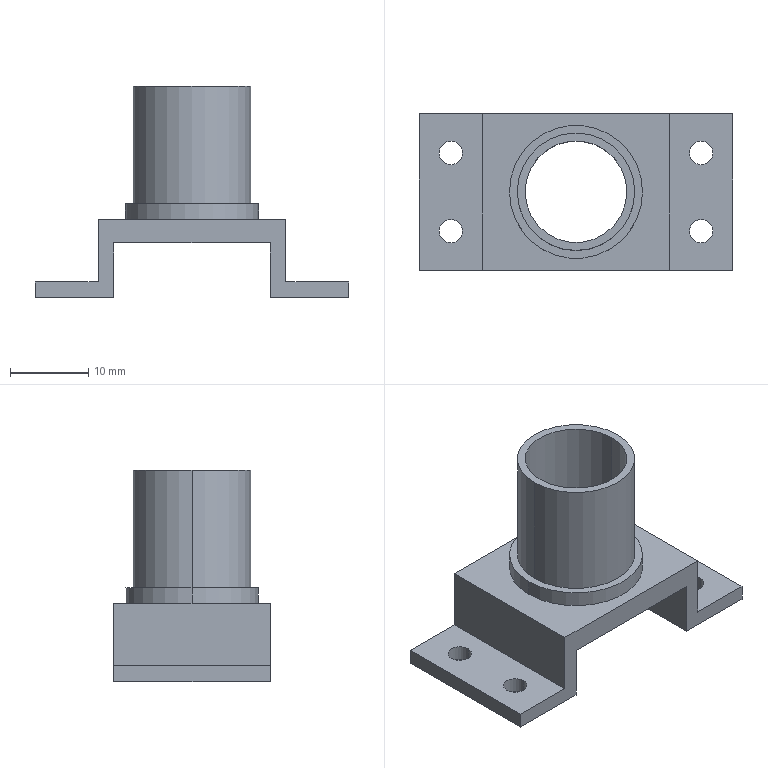Part | SolidWorks | features ICE 9, Extrusion 1 | 1 solid | 30 faces | box 40 x 20 x 27 mm | volume 3033 mm3 | plane 16 | cylinder 14 | commonest cylinder face diameters 3 x8 13 x2 15 x2 17 x2
STEP:
#1=CARTESIAN_POINT('',(14.5,-5.,-5.));
#2=VERTEX_POINT('',#1);
#3=CARTESIAN_POINT('',(17.5,-5.,-5.));
#4=VERTEX_POINT('',#3);
#5=CARTESIAN_POINT('',(16.,-5.,-5.));
#6=DIRECTION('',(0.,0.,1.));
#7=DIRECTION('',(1.,0.,0.));
#8=AXIS2_PLACEMENT_3D('',#5,#6,#7);
#9=CIRCLE('',#8,1.5);
#10=EDGE_CURVE('',#2,#4,#9,.T.);
#11=ORIENTED_EDGE('',*,*,#10,.F.);
#12=CARTESIAN_POINT('',(14.5,-5.,-3.));
#13=VERTEX_POINT('',#12);
#14=CARTESIAN_POINT('',(14.5,-5.,-5.));
#15=DIRECTION('',(0.,0.,1.));
#16=VECTOR('',#15,1000.);
#17=LINE('',#14,#16);
#18=EDGE_CURVE('',#2,#13,#17,.T.);
#19=ORIENTED_EDGE('',*,*,#18,.T.);
#20=CARTESIAN_POINT('',(17.5,-5.,-3.));
#21=VERTEX_POINT('',#20);
#22=CARTESIAN_POINT('',(16.,-5.,-3.));
#23=DIRECTION('',(0.,0.,1.));
#24=DIRECTION('',(1.,0.,0.));
#25=AXIS2_PLACEMENT_3D('',#22,#23,#24);
#26=CIRCLE('',#25,1.5);
#27=EDGE_CURVE('',#13,#21,#26,.T.);
#28=ORIENTED_EDGE('',*,*,#27,.T.);
#29=CARTESIAN_POINT('',(17.5,-5.,-5.));
#30=DIRECTION('',(0.,0.,1.));
#31=VECTOR('',#30,1000.);
#32=LINE('',#29,#31);
#33=EDGE_CURVE('',#4,#21,#32,.T.);
#34=ORIENTED_EDGE('',*,*,#33,.F.);
#35=EDGE_LOOP('',(#11,#19,#28,#34));
#36=FACE_OUTER_BOUND('',#35,.T.);
#37=CARTESIAN_POINT('',(16.,-5.,-5.));
#38=DIRECTION('',(0.,0.,1.));
#39=DIRECTION('',(1.,0.,0.));
#40=AXIS2_PLACEMENT_3D('',#37,#38,#39);
#41=CYLINDRICAL_SURFACE('',#40,1.5);
#42=ADVANCED_FACE('',(#36),#41,.F.);
#43=CARTESIAN_POINT('',(14.5,5.,-5.));
#44=VERTEX_POINT('',#43);
#45=CARTESIAN_POINT('',(17.5,5.,-5.));
#46=VERTEX_POINT('',#45);
#47=CARTESIAN_POINT('',(16.,5.,-5.));
#48=DIRECTION('',(0.,0.,1.));
#49=DIRECTION('',(1.,0.,0.));
#50=AXIS2_PLACEMENT_3D('',#47,#48,#49);
#51=CIRCLE('',#50,1.5);
#52=EDGE_CURVE('',#44,#46,#51,.T.);
#53=ORIENTED_EDGE('',*,*,#52,.F.);
#54=CARTESIAN_POINT('',(14.5,5.,-3.));
#55=VERTEX_POINT('',#54);
#56=CARTESIAN_POINT('',(14.5,5.,-5.));
#57=DIRECTION('',(0.,0.,1.));
#58=VECTOR('',#57,1000.);
#59=LINE('',#56,#58);
#60=EDGE_CURVE('',#44,#55,#59,.T.);
#61=ORIENTED_EDGE('',*,*,#60,.T.);
#62=CARTESIAN_POINT('',(17.5,5.,-3.));
#63=VERTEX_POINT('',#62);
#64=CARTESIAN_POINT('',(16.,5.,-3.));
#65=DIRECTION('',(0.,0.,1.));
#66=DIRECTION('',(1.,0.,0.));
#67=AXIS2_PLACEMENT_3D('',#64,#65,#66);
#68=CIRCLE('',#67,1.5);
#69=EDGE_CURVE('',#55,#63,#68,.T.);
#70=ORIENTED_EDGE('',*,*,#69,.T.);
#71=CARTESIAN_POINT('',(17.5,5.,-5.));
#72=DIRECTION('',(0.,0.,1.));
#73=VECTOR('',#72,1000.);
#74=LINE('',#71,#73);
#75=EDGE_CURVE('',#46,#63,#74,.T.);
#76=ORIENTED_EDGE('',*,*,#75,.F.);
#77=EDGE_LOOP('',(#53,#61,#70,#76));
#78=FACE_OUTER_BOUND('',#77,.T.);
#79=CARTESIAN_POINT('',(16.,5.,-5.));
#80=DIRECTION('',(0.,0.,1.));
#81=DIRECTION('',(1.,0.,0.));
#82=AXIS2_PLACEMENT_3D('',#79,#80,#81);
#83=CYLINDRICAL_SURFACE('',#82,1.5);
#84=ADVANCED_FACE('',(#78),#83,.F.);
#85=CARTESIAN_POINT('',(-17.5,5.,-5.));
#86=VERTEX_POINT('',#85);
#87=CARTESIAN_POINT('',(-14.5,5.,-5.));
#88=VERTEX_POINT('',#87);
#89=CARTESIAN_POINT('',(-16.,5.,-5.));
#90=DIRECTION('',(0.,0.,1.));
#91=DIRECTION('',(-1.,0.,0.));
#92=AXIS2_PLACEMENT_3D('',#89,#90,#91);
#93=CIRCLE('',#92,1.5);
#94=EDGE_CURVE('',#86,#88,#93,.T.);
#95=ORIENTED_EDGE('',*,*,#94,.F.);
#96=CARTESIAN_POINT('',(-17.5,5.,-3.));
#97=VERTEX_POINT('',#96);
#98=CARTESIAN_POINT('',(-17.5,5.,-5.));
#99=DIRECTION('',(0.,0.,1.));
#100=VECTOR('',#99,1000.);
#101=LINE('',#98,#100);
#102=EDGE_CURVE('',#86,#97,#101,.T.);
#103=ORIENTED_EDGE('',*,*,#102,.T.);
#104=CARTESIAN_POINT('',(-14.5,5.,-3.));
#105=VERTEX_POINT('',#104);
#106=CARTESIAN_POINT('',(-16.,5.,-3.));
#107=DIRECTION('',(0.,0.,1.));
#108=DIRECTION('',(-1.,0.,0.));
#109=AXIS2_PLACEMENT_3D('',#106,#107,#108);
#110=CIRCLE('',#109,1.5);
#111=EDGE_CURVE('',#97,#105,#110,.T.);
#112=ORIENTED_EDGE('',*,*,#111,.T.);
#113=CARTESIAN_POINT('',(-14.5,5.,-5.));
#114=DIRECTION('',(0.,0.,1.));
#115=VECTOR('',#114,1000.);
#116=LINE('',#113,#115);
#117=EDGE_CURVE('',#88,#105,#116,.T.);
#118=ORIENTED_EDGE('',*,*,#117,.F.);
#119=EDGE_LOOP('',(#95,#103,#112,#118));
#120=FACE_OUTER_BOUND('',#119,.T.);
#121=CARTESIAN_POINT('',(-16.,5.,-5.));
#122=DIRECTION('',(0.,0.,1.));
#123=DIRECTION('',(1.,0.,0.));
#124=AXIS2_PLACEMENT_3D('',#121,#122,#123);
#125=CYLINDRICAL_SURFACE('',#124,1.5);
#126=ADVANCED_FACE('',(#120),#125,.F.);
#127=CARTESIAN_POINT('',(-17.5,-5.,-5.));
#128=VERTEX_POINT('',#127);
#129=CARTESIAN_POINT('',(-14.5,-5.,-5.));
#130=VERTEX_POINT('',#129);
#131=CARTESIAN_POINT('',(-16.,-5.,-5.));
#132=DIRECTION('',(0.,0.,1.));
#133=DIRECTION('',(-1.,0.,0.));
#134=AXIS2_PLACEMENT_3D('',#131,#132,#133);
#135=CIRCLE('',#134,1.5);
#136=EDGE_CURVE('',#128,#130,#135,.T.);
#137=ORIENTED_EDGE('',*,*,#136,.F.);
#138=CARTESIAN_POINT('',(-17.5,-5.,-3.));
#139=VERTEX_POINT('',#138);
#140=CARTESIAN_POINT('',(-17.5,-5.,-5.));
#141=DIRECTION('',(0.,0.,1.));
#142=VECTOR('',#141,1000.);
#143=LINE('',#140,#142);
#144=EDGE_CURVE('',#128,#139,#143,.T.);
#145=ORIENTED_EDGE('',*,*,#144,.T.);
#146=CARTESIAN_POINT('',(-14.5,-5.,-3.));
#147=VERTEX_POINT('',#146);
#148=CARTESIAN_POINT('',(-16.,-5.,-3.));
#149=DIRECTION('',(0.,0.,1.));
#150=DIRECTION('',(-1.,0.,0.));
#151=AXIS2_PLACEMENT_3D('',#148,#149,#150);
#152=CIRCLE('',#151,1.5);
#153=EDGE_CURVE('',#139,#147,#152,.T.);
#154=ORIENTED_EDGE('',*,*,#153,.T.);
#155=CARTESIAN_POINT('',(-14.5,-5.,-5.));
#156=DIRECTION('',(0.,0.,1.));
#157=VECTOR('',#156,1000.);
#158=LINE('',#155,#157);
#159=EDGE_CURVE('',#130,#147,#158,.T.);
#160=ORIENTED_EDGE('',*,*,#159,.F.);
#161=EDGE_LOOP('',(#137,#145,#154,#160));
#162=FACE_OUTER_BOUND('',#161,.T.);
#163=CARTESIAN_POINT('',(-16.,-5.,-5.));
#164=DIRECTION('',(0.,0.,1.));
#165=DIRECTION('',(1.,0.,0.));
#166=AXIS2_PLACEMENT_3D('',#163,#164,#165);
#167=CYLINDRICAL_SURFACE('',#166,1.5);
#168=ADVANCED_FACE('',(#162),#167,.F.);
#169=CARTESIAN_POINT('',(-8.5,0.,5.));
#170=VERTEX_POINT('',#169);
#171=CARTESIAN_POINT('',(8.5,0.,5.));
#172=VERTEX_POINT('',#171);
#173=CARTESIAN_POINT('',(0.,0.,5.));
#174=DIRECTION('',(0.,0.,-1.));
#175=DIRECTION('',(-1.,0.,0.));
#176=AXIS2_PLACEMENT_3D('',#173,#174,#175);
#177=CIRCLE('',#176,8.5);
#178=EDGE_CURVE('',#170,#172,#177,.T.);
#179=ORIENTED_EDGE('',*,*,#178,.F.);
#180=CARTESIAN_POINT('',(-8.5,0.,7.));
#181=VERTEX_POINT('',#180);
#182=CARTESIAN_POINT('',(-8.5,0.,5.));
#183=DIRECTION('',(0.,0.,1.));
#184=VECTOR('',#183,1000.);
#185=LINE('',#182,#184);
#186=EDGE_CURVE('',#170,#181,#185,.T.);
#187=ORIENTED_EDGE('',*,*,#186,.T.);
#188=CARTESIAN_POINT('',(8.5,0.,7.));
#189=VERTEX_POINT('',#188);
#190=CARTESIAN_POINT('',(0.,0.,7.));
#191=DIRECTION('',(0.,0.,-1.));
#192=DIRECTION('',(-1.,0.,0.));
#193=AXIS2_PLACEMENT_3D('',#190,#191,#192);
#194=CIRCLE('',#193,8.5);
#195=EDGE_CURVE('',#181,#189,#194,.T.);
#196=ORIENTED_EDGE('',*,*,#195,.T.);
#197=CARTESIAN_POINT('',(8.5,0.,5.));
#198=DIRECTION('',(0.,0.,1.));
#199=VECTOR('',#198,1000.);
#200=LINE('',#197,#199);
#201=EDGE_CURVE('',#172,#189,#200,.T.);
#202=ORIENTED_EDGE('',*,*,#201,.F.);
#203=EDGE_LOOP('',(#179,#187,#196,#202));
#204=FACE_OUTER_BOUND('',#203,.T.);
#205=CARTESIAN_POINT('',(0.,0.,5.));
#206=DIRECTION('',(0.,0.,1.));
#207=DIRECTION('',(1.,0.,0.));
#208=AXIS2_PLACEMENT_3D('',#205,#206,#207);
#209=CYLINDRICAL_SURFACE('',#208,8.5);
#210=ADVANCED_FACE('',(#204),#209,.T.);
#211=CARTESIAN_POINT('',(7.5,0.,22.));
#212=VERTEX_POINT('',#211);
#213=CARTESIAN_POINT('',(-7.5,0.,22.));
#214=VERTEX_POINT('',#213);
#215=CARTESIAN_POINT('',(0.,0.,22.));
#216=DIRECTION('',(0.,0.,1.));
#217=DIRECTION('',(1.,0.,0.));
#218=AXIS2_PLACEMENT_3D('',#215,#216,#217);
#219=CIRCLE('',#218,7.5);
#220=EDGE_CURVE('',#212,#214,#219,.T.);
#221=ORIENTED_EDGE('',*,*,#220,.F.);
#222=CARTESIAN_POINT('',(7.5,0.,7.));
#223=VERTEX_POINT('',#222);
#224=CARTESIAN_POINT('',(7.5,0.,22.));
#225=DIRECTION('',(0.,0.,-1.));
#226=VECTOR('',#225,1000.);
#227=LINE('',#224,#226);
#228=EDGE_CURVE('',#212,#223,#227,.T.);
#229=ORIENTED_EDGE('',*,*,#228,.T.);
#230=CARTESIAN_POINT('',(-7.5,0.,7.));
#231=VERTEX_POINT('',#230);
#232=CARTESIAN_POINT('',(0.,0.,7.));
#233=DIRECTION('',(0.,0.,-1.));
#234=DIRECTION('',(-1.,0.,0.));
#235=AXIS2_PLACEMENT_3D('',#232,#233,#234);
#236=CIRCLE('',#235,7.5);
#237=EDGE_CURVE('',#231,#223,#236,.T.);
#238=ORIENTED_EDGE('',*,*,#237,.F.);
#239=CARTESIAN_POINT('',(-7.5,0.,22.));
#240=DIRECTION('',(0.,0.,-1.));
#241=VECTOR('',#240,1000.);
#242=LINE('',#239,#241);
#243=EDGE_CURVE('',#214,#231,#242,.T.);
#244=ORIENTED_EDGE('',*,*,#243,.F.);
#245=EDGE_LOOP('',(#221,#229,#238,#244));
#246=FACE_OUTER_BOUND('',#245,.T.);
#247=CARTESIAN_POINT('',(0.,0.,22.));
#248=DIRECTION('',(0.,0.,-1.));
#249=DIRECTION('',(-1.,0.,0.));
#250=AXIS2_PLACEMENT_3D('',#247,#248,#249);
#251=CYLINDRICAL_SURFACE('',#250,7.5);
#252=ADVANCED_FACE('',(#246),#251,.T.);
#253=CARTESIAN_POINT('',(-6.5,0.,22.));
#254=VERTEX_POINT('',#253);
#255=CARTESIAN_POINT('',(6.5,0.,22.));
#256=VERTEX_POINT('',#255);
#257=CARTESIAN_POINT('',(0.,0.,22.));
#258=DIRECTION('',(0.,0.,1.));
#259=DIRECTION('',(1.,0.,0.));
#260=AXIS2_PLACEMENT_3D('',#257,#258,#259);
#261=CIRCLE('',#260,6.5);
#262=EDGE_CURVE('',#254,#256,#261,.T.);
#263=ORIENTED_EDGE('',*,*,#262,.T.);
#264=CARTESIAN_POINT('',(6.5,0.,2.));
#265=VERTEX_POINT('',#264);
#266=CARTESIAN_POINT('',(6.5,0.,22.));
#267=DIRECTION('',(0.,0.,-1.));
#268=VECTOR('',#267,1000.);
#269=LINE('',#266,#268);
#270=EDGE_CURVE('',#256,#265,#269,.T.);
#271=ORIENTED_EDGE('',*,*,#270,.T.);
#272=CARTESIAN_POINT('',(-6.5,0.,2.));
#273=VERTEX_POINT('',#272);
#274=CARTESIAN_POINT('',(0.,0.,2.));
#275=DIRECTION('',(0.,0.,-1.));
#276=DIRECTION('',(-1.,0.,0.));
#277=AXIS2_PLACEMENT_3D('',#274,#275,#276);
#278=CIRCLE('',#277,6.5);
#279=EDGE_CURVE('',#265,#273,#278,.T.);
#280=ORIENTED_EDGE('',*,*,#279,.T.);
#281=CARTESIAN_POINT('',(-6.5,0.,22.));
#282=DIRECTION('',(0.,0.,-1.));
#283=VECTOR('',#282,1000.);
#284=LINE('',#281,#283);
#285=EDGE_CURVE('',#254,#273,#284,.T.);
#286=ORIENTED_EDGE('',*,*,#285,.F.);
#287=EDGE_LOOP('',(#263,#271,#280,#286));
#288=FACE_OUTER_BOUND('',#287,.T.);
#289=CARTESIAN_POINT('',(0.,0.,22.));
#290=DIRECTION('',(0.,0.,-1.));
#291=DIRECTION('',(-1.,0.,0.));
#292=AXIS2_PLACEMENT_3D('',#289,#290,#291);
#293=CYLINDRICAL_SURFACE('',#292,6.5);
#294=ADVANCED_FACE('',(#288),#293,.F.);
#295=CARTESIAN_POINT('',(-16.,5.,-5.));
#296=DIRECTION('',(0.,0.,1.));
#297=DIRECTION('',(-1.,0.,0.));
#298=AXIS2_PLACEMENT_3D('',#295,#296,#297);
#299=CIRCLE('',#298,1.5);
#300=EDGE_CURVE('',#88,#86,#299,.T.);
#301=ORIENTED_EDGE('',*,*,#300,.T.);
#302=ORIENTED_EDGE('',*,*,#94,.T.);
#303=EDGE_LOOP('',(#301,#302));
#304=FACE_BOUND('',#303,.T.);
#305=CARTESIAN_POINT('',(-16.,-5.,-5.));
#306=DIRECTION('',(0.,0.,1.));
#307=DIRECTION('',(-1.,0.,0.));
#308=AXIS2_PLACEMENT_3D('',#305,#306,#307);
#309=CIRCLE('',#308,1.5);
#310=EDGE_CURVE('',#130,#128,#309,.T.);
#311=ORIENTED_EDGE('',*,*,#310,.T.);
#312=ORIENTED_EDGE('',*,*,#136,.T.);
#313=EDGE_LOOP('',(#311,#312));
#314=FACE_BOUND('',#313,.T.);
#315=CARTESIAN_POINT('',(-10.,10.,-5.));
#316=VERTEX_POINT('',#315);
#317=CARTESIAN_POINT('',(-10.,-10.,-5.));
#318=VERTEX_POINT('',#317);
#319=CARTESIAN_POINT('',(-10.,10.,-5.));
#320=DIRECTION('',(0.,-1.,0.));
#321=VECTOR('',#320,1000.);
#322=LINE('',#319,#321);
#323=EDGE_CURVE('',#316,#318,#322,.T.);
#324=ORIENTED_EDGE('',*,*,#323,.T.);
#325=CARTESIAN_POINT('',(-20.,-10.,-5.));
#326=VERTEX_POINT('',#325);
#327=CARTESIAN_POINT('',(-15.,-10.,-5.));
#328=DIRECTION('',(-1.,0.,0.));
#329=VECTOR('',#328,1000.);
#330=LINE('',#327,#329);
#331=EDGE_CURVE('',#318,#326,#330,.T.);
#332=ORIENTED_EDGE('',*,*,#331,.T.);
#333=CARTESIAN_POINT('',(-20.,10.,-5.));
#334=VERTEX_POINT('',#333);
#335=CARTESIAN_POINT('',(-20.,10.,-5.));
#336=DIRECTION('',(0.,1.,0.));
#337=VECTOR('',#336,1000.);
#338=LINE('',#335,#337);
#339=EDGE_CURVE('',#326,#334,#338,.T.);
#340=ORIENTED_EDGE('',*,*,#339,.T.);
#341=CARTESIAN_POINT('',(-15.,10.,-5.));
#342=DIRECTION('',(1.,0.,0.));
#343=VECTOR('',#342,1000.);
#344=LINE('',#341,#343);
#345=EDGE_CURVE('',#334,#316,#344,.T.);
#346=ORIENTED_EDGE('',*,*,#345,.T.);
#347=EDGE_LOOP('',(#324,#332,#340,#346));
#348=FACE_OUTER_BOUND('',#347,.T.);
#349=CARTESIAN_POINT('',(0.,0.,-5.));
#350=DIRECTION('',(0.,0.,-1.));
#351=DIRECTION('',(-1.,0.,0.));
#352=AXIS2_PLACEMENT_3D('',#349,#350,#351);
#353=PLANE('',#352);
#354=ADVANCED_FACE('',(#304,#314,#348),#353,.T.);
#355=CARTESIAN_POINT('',(12.,-10.,5.));
#356=VERTEX_POINT('',#355);
#357=CARTESIAN_POINT('',(-12.,-10.,5.));
#358=VERTEX_POINT('',#357);
#359=CARTESIAN_POINT('',(-15.,-10.,5.));
#360=DIRECTION('',(-1.,0.,0.));
#361=VECTOR('',#360,1000.);
#362=LINE('',#359,#361);
#363=EDGE_CURVE('',#356,#358,#362,.T.);
#364=ORIENTED_EDGE('',*,*,#363,.T.);
#365=CARTESIAN_POINT('',(-12.,-10.,-3.));
#366=VERTEX_POINT('',#365);
#367=CARTESIAN_POINT('',(-12.,-10.,-3.));
#368=DIRECTION('',(0.,0.,1.));
#369=VECTOR('',#368,1000.);
#370=LINE('',#367,#369);
#371=EDGE_CURVE('',#366,#358,#370,.T.);
#372=ORIENTED_EDGE('',*,*,#371,.F.);
#373=CARTESIAN_POINT('',(-20.,-10.,-3.));
#374=VERTEX_POINT('',#373);
#375=CARTESIAN_POINT('',(-15.,-10.,-3.));
#376=DIRECTION('',(-1.,0.,0.));
#377=VECTOR('',#376,1000.);
#378=LINE('',#375,#377);
#379=EDGE_CURVE('',#366,#374,#378,.T.);
#380=ORIENTED_EDGE('',*,*,#379,.T.);
#381=CARTESIAN_POINT('',(-20.,-10.,-3.));
#382=DIRECTION('',(0.,0.,-1.));
#383=VECTOR('',#382,1000.);
#384=LINE('',#381,#383);
#385=EDGE_CURVE('',#374,#326,#384,.T.);
#386=ORIENTED_EDGE('',*,*,#385,.T.);
#387=ORIENTED_EDGE('',*,*,#331,.F.);
#388=CARTESIAN_POINT('',(-10.,-10.,2.));
#389=VERTEX_POINT('',#388);
#390=CARTESIAN_POINT('',(-10.,-10.,-5.));
#391=DIRECTION('',(0.,0.,-1.));
#392=VECTOR('',#391,1000.);
#393=LINE('',#390,#392);
#394=EDGE_CURVE('',#389,#318,#393,.T.);
#395=ORIENTED_EDGE('',*,*,#394,.F.);
#396=CARTESIAN_POINT('',(10.,-10.,2.));
#397=VERTEX_POINT('',#396);
#398=CARTESIAN_POINT('',(-10.,-10.,2.));
#399=DIRECTION('',(-1.,0.,0.));
#400=VECTOR('',#399,1000.);
#401=LINE('',#398,#400);
#402=EDGE_CURVE('',#397,#389,#401,.T.);
#403=ORIENTED_EDGE('',*,*,#402,.F.);
#404=CARTESIAN_POINT('',(10.,-10.,-5.));
#405=VERTEX_POINT('',#404);
#406=CARTESIAN_POINT('',(10.,-10.,-5.));
#407=DIRECTION('',(0.,0.,1.));
#408=VECTOR('',#407,1000.);
#409=LINE('',#406,#408);
#410=EDGE_CURVE('',#405,#397,#409,.T.);
#411=ORIENTED_EDGE('',*,*,#410,.F.);
#412=CARTESIAN_POINT('',(20.,-10.,-5.));
#413=VERTEX_POINT('',#412);
#414=CARTESIAN_POINT('',(-15.,-10.,-5.));
#415=DIRECTION('',(-1.,0.,0.));
#416=VECTOR('',#415,1000.);
#417=LINE('',#414,#416);
#418=EDGE_CURVE('',#413,#405,#417,.T.);
#419=ORIENTED_EDGE('',*,*,#418,.F.);
#420=CARTESIAN_POINT('',(20.,-10.,-3.));
#421=VERTEX_POINT('',#420);
#422=CARTESIAN_POINT('',(20.,-10.,-3.));
#423=DIRECTION('',(0.,0.,-1.));
#424=VECTOR('',#423,1000.);
#425=LINE('',#422,#424);
#426=EDGE_CURVE('',#421,#413,#425,.T.);
#427=ORIENTED_EDGE('',*,*,#426,.F.);
#428=CARTESIAN_POINT('',(12.,-10.,-3.));
#429=VERTEX_POINT('',#428);
#430=CARTESIAN_POINT('',(15.,-10.,-3.));
#431=DIRECTION('',(-1.,0.,0.));
#432=VECTOR('',#431,1000.);
#433=LINE('',#430,#432);
#434=EDGE_CURVE('',#421,#429,#433,.T.);
#435=ORIENTED_EDGE('',*,*,#434,.T.);
#436=CARTESIAN_POINT('',(12.,-10.,-3.));
#437=DIRECTION('',(0.,0.,1.));
#438=VECTOR('',#437,1000.);
#439=LINE('',#436,#438);
#440=EDGE_CURVE('',#429,#356,#439,.T.);
#441=ORIENTED_EDGE('',*,*,#440,.T.);
#442=EDGE_LOOP('',(#364,#372,#380,#386,#387,#395,#403,#411,#419,#427,#435,#441));
#443=FACE_OUTER_BOUND('',#442,.T.);
#444=CARTESIAN_POINT('',(-15.,-10.,-5.));
#445=DIRECTION('',(0.,1.,0.));
#446=DIRECTION('',(0.,0.,1.));
#447=AXIS2_PLACEMENT_3D('',#444,#445,#446);
#448=PLANE('',#447);
#449=ADVANCED_FACE('',(#443),#448,.F.);
#450=CARTESIAN_POINT('',(-20.,10.,-3.));
#451=VERTEX_POINT('',#450);
#452=CARTESIAN_POINT('',(-12.,10.,-3.));
#453=VERTEX_POINT('',#452);
#454=CARTESIAN_POINT('',(-15.,10.,-3.));
#455=DIRECTION('',(1.,0.,0.));
#456=VECTOR('',#455,1000.);
#457=LINE('',#454,#456);
#458=EDGE_CURVE('',#451,#453,#457,.T.);
#459=ORIENTED_EDGE('',*,*,#458,.T.);
#460=CARTESIAN_POINT('',(-12.,10.,5.));
#461=VERTEX_POINT('',#460);
#462=CARTESIAN_POINT('',(-12.,10.,-3.));
#463=DIRECTION('',(0.,0.,1.));
#464=VECTOR('',#463,1000.);
#465=LINE('',#462,#464);
#466=EDGE_CURVE('',#453,#461,#465,.T.);
#467=ORIENTED_EDGE('',*,*,#466,.T.);
#468=CARTESIAN_POINT('',(12.,10.,5.));
#469=VERTEX_POINT('',#468);
#470=CARTESIAN_POINT('',(-15.,10.,5.));
#471=DIRECTION('',(1.,0.,0.));
#472=VECTOR('',#471,1000.);
#473=LINE('',#470,#472);
#474=EDGE_CURVE('',#461,#469,#473,.T.);
#475=ORIENTED_EDGE('',*,*,#474,.T.);
#476=CARTESIAN_POINT('',(12.,10.,-3.));
#477=VERTEX_POINT('',#476);
#478=CARTESIAN_POINT('',(12.,10.,-3.));
#479=DIRECTION('',(0.,0.,1.));
#480=VECTOR('',#479,1000.);
#481=LINE('',#478,#480);
#482=EDGE_CURVE('',#477,#469,#481,.T.);
#483=ORIENTED_EDGE('',*,*,#482,.F.);
#484=CARTESIAN_POINT('',(20.,10.,-3.));
#485=VERTEX_POINT('',#484);
#486=CARTESIAN_POINT('',(15.,10.,-3.));
#487=DIRECTION('',(1.,0.,0.));
#488=VECTOR('',#487,1000.);
#489=LINE('',#486,#488);
#490=EDGE_CURVE('',#477,#485,#489,.T.);
#491=ORIENTED_EDGE('',*,*,#490,.T.);
#492=CARTESIAN_POINT('',(20.,10.,-5.));
#493=VERTEX_POINT('',#492);
#494=CARTESIAN_POINT('',(20.,10.,-3.));
#495=DIRECTION('',(0.,0.,-1.));
#496=VECTOR('',#495,1000.);
#497=LINE('',#494,#496);
#498=EDGE_CURVE('',#485,#493,#497,.T.);
#499=ORIENTED_EDGE('',*,*,#498,.T.);
#500=CARTESIAN_POINT('',(10.,10.,-5.));
#501=VERTEX_POINT('',#500);
#502=CARTESIAN_POINT('',(-15.,10.,-5.));
#503=DIRECTION('',(1.,0.,0.));
#504=VECTOR('',#503,1000.);
#505=LINE('',#502,#504);
#506=EDGE_CURVE('',#501,#493,#505,.T.);
#507=ORIENTED_EDGE('',*,*,#506,.F.);
#508=CARTESIAN_POINT('',(10.,10.,2.));
#509=VERTEX_POINT('',#508);
#510=CARTESIAN_POINT('',(10.,10.,-5.));
#511=DIRECTION('',(0.,0.,1.));
#512=VECTOR('',#511,1000.);
#513=LINE('',#510,#512);
#514=EDGE_CURVE('',#501,#509,#513,.T.);
#515=ORIENTED_EDGE('',*,*,#514,.T.);
#516=CARTESIAN_POINT('',(-10.,10.,2.));
#517=VERTEX_POINT('',#516);
#518=CARTESIAN_POINT('',(-10.,10.,2.));
#519=DIRECTION('',(-1.,0.,0.));
#520=VECTOR('',#519,1000.);
#521=LINE('',#518,#520);
#522=EDGE_CURVE('',#509,#517,#521,.T.);
#523=ORIENTED_EDGE('',*,*,#522,.T.);
#524=CARTESIAN_POINT('',(-10.,10.,-5.));
#525=DIRECTION('',(0.,0.,-1.));
#526=VECTOR('',#525,1000.);
#527=LINE('',#524,#526);
#528=EDGE_CURVE('',#517,#316,#527,.T.);
#529=ORIENTED_EDGE('',*,*,#528,.T.);
#530=ORIENTED_EDGE('',*,*,#345,.F.);
#531=CARTESIAN_POINT('',(-20.,10.,-3.));
#532=DIRECTION('',(0.,0.,-1.));
#533=VECTOR('',#532,1000.);
#534=LINE('',#531,#533);
#535=EDGE_CURVE('',#451,#334,#534,.T.);
#536=ORIENTED_EDGE('',*,*,#535,.F.);
#537=EDGE_LOOP('',(#459,#467,#475,#483,#491,#499,#507,#515,#523,#529,#530,#536));
#538=FACE_OUTER_BOUND('',#537,.T.);
#539=CARTESIAN_POINT('',(-15.,10.,-5.));
#540=DIRECTION('',(0.,-1.,0.));
#541=DIRECTION('',(0.,0.,-1.));
#542=AXIS2_PLACEMENT_3D('',#539,#540,#541);
#543=PLANE('',#542);
#544=ADVANCED_FACE('',(#538),#543,.F.);
#545=CARTESIAN_POINT('',(16.,-5.,-5.));
#546=DIRECTION('',(0.,0.,1.));
#547=DIRECTION('',(1.,0.,0.));
#548=AXIS2_PLACEMENT_3D('',#545,#546,#547);
#549=CIRCLE('',#548,1.5);
#550=EDGE_CURVE('',#4,#2,#549,.T.);
#551=ORIENTED_EDGE('',*,*,#550,.T.);
#552=ORIENTED_EDGE('',*,*,#10,.T.);
#553=EDGE_LOOP('',(#551,#552));
#554=FACE_BOUND('',#553,.T.);
#555=CARTESIAN_POINT('',(16.,5.,-5.));
#556=DIRECTION('',(0.,0.,1.));
#557=DIRECTION('',(1.,0.,0.));
#558=AXIS2_PLACEMENT_3D('',#555,#556,#557);
#559=CIRCLE('',#558,1.5);
#560=EDGE_CURVE('',#46,#44,#559,.T.);
#561=ORIENTED_EDGE('',*,*,#560,.T.);
#562=ORIENTED_EDGE('',*,*,#52,.T.);
#563=EDGE_LOOP('',(#561,#562));
#564=FACE_BOUND('',#563,.T.);
#565=CARTESIAN_POINT('',(10.,10.,-5.));
#566=DIRECTION('',(0.,-1.,0.));
#567=VECTOR('',#566,1000.);
#568=LINE('',#565,#567);
#569=EDGE_CURVE('',#501,#405,#568,.T.);
#570=ORIENTED_EDGE('',*,*,#569,.F.);
#571=ORIENTED_EDGE('',*,*,#506,.T.);
#572=CARTESIAN_POINT('',(20.,10.,-5.));
#573=DIRECTION('',(0.,-1.,0.));
#574=VECTOR('',#573,1000.);
#575=LINE('',#572,#574);
#576=EDGE_CURVE('',#493,#413,#575,.T.);
#577=ORIENTED_EDGE('',*,*,#576,.T.);
#578=ORIENTED_EDGE('',*,*,#418,.T.);
#579=EDGE_LOOP('',(#570,#571,#577,#578));
#580=FACE_OUTER_BOUND('',#579,.T.);
#581=CARTESIAN_POINT('',(0.,0.,-5.));
#582=DIRECTION('',(0.,0.,-1.));
#583=DIRECTION('',(-1.,0.,0.));
#584=AXIS2_PLACEMENT_3D('',#581,#582,#583);
#585=PLANE('',#584);
#586=ADVANCED_FACE('',(#554,#564,#580),#585,.T.);
#587=CARTESIAN_POINT('',(0.,0.,5.));
#588=DIRECTION('',(0.,0.,-1.));
#589=DIRECTION('',(-1.,0.,0.));
#590=AXIS2_PLACEMENT_3D('',#587,#588,#589);
#591=CIRCLE('',#590,8.5);
#592=EDGE_CURVE('',#172,#170,#591,.T.);
#593=ORIENTED_EDGE('',*,*,#592,.T.);
#594=ORIENTED_EDGE('',*,*,#178,.T.);
#595=EDGE_LOOP('',(#593,#594));
#596=FACE_BOUND('',#595,.T.);
#597=ORIENTED_EDGE('',*,*,#474,.F.);
#598=CARTESIAN_POINT('',(-12.,10.,5.));
#599=DIRECTION('',(0.,1.,0.));
#600=VECTOR('',#599,1000.);
#601=LINE('',#598,#600);
#602=EDGE_CURVE('',#358,#461,#601,.T.);
#603=ORIENTED_EDGE('',*,*,#602,.F.);
#604=ORIENTED_EDGE('',*,*,#363,.F.);
#605=CARTESIAN_POINT('',(12.,10.,5.));
#606=DIRECTION('',(0.,-1.,0.));
#607=VECTOR('',#606,1000.);
#608=LINE('',#605,#607);
#609=EDGE_CURVE('',#469,#356,#608,.T.);
#610=ORIENTED_EDGE('',*,*,#609,.F.);
#611=EDGE_LOOP('',(#597,#603,#604,#610));
#612=FACE_OUTER_BOUND('',#611,.T.);
#613=CARTESIAN_POINT('',(0.,0.,5.));
#614=DIRECTION('',(0.,0.,-1.));
#615=DIRECTION('',(-1.,0.,0.));
#616=AXIS2_PLACEMENT_3D('',#613,#614,#615);
#617=PLANE('',#616);
#618=ADVANCED_FACE('',(#596,#612),#617,.F.);
#619=ORIENTED_EDGE('',*,*,#270,.F.);
#620=CARTESIAN_POINT('',(0.,0.,22.));
#621=DIRECTION('',(0.,0.,1.));
#622=DIRECTION('',(1.,0.,0.));
#623=AXIS2_PLACEMENT_3D('',#620,#621,#622);
#624=CIRCLE('',#623,6.5);
#625=EDGE_CURVE('',#256,#254,#624,.T.);
#626=ORIENTED_EDGE('',*,*,#625,.T.);
#627=ORIENTED_EDGE('',*,*,#285,.T.);
#628=CARTESIAN_POINT('',(0.,0.,2.));
#629=DIRECTION('',(0.,0.,-1.));
#630=DIRECTION('',(-1.,0.,0.));
#631=AXIS2_PLACEMENT_3D('',#628,#629,#630);
#632=CIRCLE('',#631,6.5);
#633=EDGE_CURVE('',#273,#265,#632,.T.);
#634=ORIENTED_EDGE('',*,*,#633,.T.);
#635=EDGE_LOOP('',(#619,#626,#627,#634));
#636=FACE_OUTER_BOUND('',#635,.T.);
#637=CARTESIAN_POINT('',(0.,0.,22.));
#638=DIRECTION('',(0.,0.,-1.));
#639=DIRECTION('',(-1.,0.,0.));
#640=AXIS2_PLACEMENT_3D('',#637,#638,#639);
#641=CYLINDRICAL_SURFACE('',#640,6.5);
#642=ADVANCED_FACE('',(#636),#641,.F.);
#643=ORIENTED_EDGE('',*,*,#228,.F.);
#644=CARTESIAN_POINT('',(0.,0.,22.));
#645=DIRECTION('',(0.,0.,1.));
#646=DIRECTION('',(1.,0.,0.));
#647=AXIS2_PLACEMENT_3D('',#644,#645,#646);
#648=CIRCLE('',#647,7.5);
#649=EDGE_CURVE('',#214,#212,#648,.T.);
#650=ORIENTED_EDGE('',*,*,#649,.F.);
#651=ORIENTED_EDGE('',*,*,#243,.T.);
#652=CARTESIAN_POINT('',(0.,0.,7.));
#653=DIRECTION('',(0.,0.,-1.));
#654=DIRECTION('',(-1.,0.,0.));
#655=AXIS2_PLACEMENT_3D('',#652,#653,#654);
#656=CIRCLE('',#655,7.5);
#657=EDGE_CURVE('',#223,#231,#656,.T.);
#658=ORIENTED_EDGE('',*,*,#657,.F.);
#659=EDGE_LOOP('',(#643,#650,#651,#658));
#660=FACE_OUTER_BOUND('',#659,.T.);
#661=CARTESIAN_POINT('',(0.,0.,22.));
#662=DIRECTION('',(0.,0.,-1.));
#663=DIRECTION('',(-1.,0.,0.));
#664=AXIS2_PLACEMENT_3D('',#661,#662,#663);
#665=CYLINDRICAL_SURFACE('',#664,7.5);
#666=ADVANCED_FACE('',(#660),#665,.T.);
#667=ORIENTED_EDGE('',*,*,#649,.T.);
#668=ORIENTED_EDGE('',*,*,#220,.T.);
#669=EDGE_LOOP('',(#667,#668));
#670=FACE_OUTER_BOUND('',#669,.T.);
#671=ORIENTED_EDGE('',*,*,#262,.F.);
#672=ORIENTED_EDGE('',*,*,#625,.F.);
#673=EDGE_LOOP('',(#671,#672));
#674=FACE_BOUND('',#673,.T.);
#675=CARTESIAN_POINT('',(0.,0.,22.));
#676=DIRECTION('',(0.,0.,1.));
#677=DIRECTION('',(1.,0.,0.));
#678=AXIS2_PLACEMENT_3D('',#675,#676,#677);
#679=PLANE('',#678);
#680=ADVANCED_FACE('',(#670,#674),#679,.T.);
#681=CARTESIAN_POINT('',(0.,0.,7.));
#682=DIRECTION('',(0.,0.,-1.));
#683=DIRECTION('',(-1.,0.,0.));
#684=AXIS2_PLACEMENT_3D('',#681,#682,#683);
#685=CIRCLE('',#684,8.5);
#686=EDGE_CURVE('',#189,#181,#685,.T.);
#687=ORIENTED_EDGE('',*,*,#686,.F.);
#688=ORIENTED_EDGE('',*,*,#195,.F.);
#689=EDGE_LOOP('',(#687,#688));
#690=FACE_OUTER_BOUND('',#689,.T.);
#691=ORIENTED_EDGE('',*,*,#237,.T.);
#692=ORIENTED_EDGE('',*,*,#657,.T.);
#693=EDGE_LOOP('',(#691,#692));
#694=FACE_BOUND('',#693,.T.);
#695=CARTESIAN_POINT('',(0.,0.,7.));
#696=DIRECTION('',(0.,0.,-1.));
#697=DIRECTION('',(-1.,0.,0.));
#698=AXIS2_PLACEMENT_3D('',#695,#696,#697);
#699=PLANE('',#698);
#700=ADVANCED_FACE('',(#690,#694),#699,.F.);
#701=ORIENTED_EDGE('',*,*,#186,.F.);
#702=ORIENTED_EDGE('',*,*,#592,.F.);
#703=ORIENTED_EDGE('',*,*,#201,.T.);
#704=ORIENTED_EDGE('',*,*,#686,.T.);
#705=EDGE_LOOP('',(#701,#702,#703,#704));
#706=FACE_OUTER_BOUND('',#705,.T.);
#707=CARTESIAN_POINT('',(0.,0.,5.));
#708=DIRECTION('',(0.,0.,1.));
#709=DIRECTION('',(1.,0.,0.));
#710=AXIS2_PLACEMENT_3D('',#707,#708,#709);
#711=CYLINDRICAL_SURFACE('',#710,8.5);
#712=ADVANCED_FACE('',(#706),#711,.T.);
#713=ORIENTED_EDGE('',*,*,#394,.T.);
#714=ORIENTED_EDGE('',*,*,#323,.F.);
#715=ORIENTED_EDGE('',*,*,#528,.F.);
#716=CARTESIAN_POINT('',(-10.,10.,2.));
#717=DIRECTION('',(0.,-1.,0.));
#718=VECTOR('',#717,1000.);
#719=LINE('',#716,#718);
#720=EDGE_CURVE('',#517,#389,#719,.T.);
#721=ORIENTED_EDGE('',*,*,#720,.T.);
#722=EDGE_LOOP('',(#713,#714,#715,#721));
#723=FACE_OUTER_BOUND('',#722,.T.);
#724=CARTESIAN_POINT('',(-10.,10.,-5.));
#725=DIRECTION('',(-1.,0.,0.));
#726=DIRECTION('',(0.,0.,1.));
#727=AXIS2_PLACEMENT_3D('',#724,#725,#726);
#728=PLANE('',#727);
#729=ADVANCED_FACE('',(#723),#728,.F.);
#730=ORIENTED_EDGE('',*,*,#633,.F.);
#731=ORIENTED_EDGE('',*,*,#279,.F.);
#732=EDGE_LOOP('',(#730,#731));
#733=FACE_BOUND('',#732,.T.);
#734=ORIENTED_EDGE('',*,*,#402,.T.);
#735=ORIENTED_EDGE('',*,*,#720,.F.);
#736=ORIENTED_EDGE('',*,*,#522,.F.);
#737=CARTESIAN_POINT('',(10.,10.,2.));
#738=DIRECTION('',(0.,-1.,0.));
#739=VECTOR('',#738,1000.);
#740=LINE('',#737,#739);
#741=EDGE_CURVE('',#509,#397,#740,.T.);
#742=ORIENTED_EDGE('',*,*,#741,.T.);
#743=EDGE_LOOP('',(#734,#735,#736,#742));
#744=FACE_OUTER_BOUND('',#743,.T.);
#745=CARTESIAN_POINT('',(-10.,10.,2.));
#746=DIRECTION('',(0.,0.,1.));
#747=DIRECTION('',(1.,0.,0.));
#748=AXIS2_PLACEMENT_3D('',#745,#746,#747);
#749=PLANE('',#748);
#750=ADVANCED_FACE('',(#733,#744),#749,.F.);
#751=ORIENTED_EDGE('',*,*,#410,.T.);
#752=ORIENTED_EDGE('',*,*,#741,.F.);
#753=ORIENTED_EDGE('',*,*,#514,.F.);
#754=ORIENTED_EDGE('',*,*,#569,.T.);
#755=EDGE_LOOP('',(#751,#752,#753,#754));
#756=FACE_OUTER_BOUND('',#755,.T.);
#757=CARTESIAN_POINT('',(10.,10.,-5.));
#758=DIRECTION('',(1.,0.,0.));
#759=DIRECTION('',(0.,0.,-1.));
#760=AXIS2_PLACEMENT_3D('',#757,#758,#759);
#761=PLANE('',#760);
#762=ADVANCED_FACE('',(#756),#761,.F.);
#763=ORIENTED_EDGE('',*,*,#576,.F.);
#764=ORIENTED_EDGE('',*,*,#498,.F.);
#765=CARTESIAN_POINT('',(20.,10.,-3.));
#766=DIRECTION('',(0.,-1.,0.));
#767=VECTOR('',#766,1000.);
#768=LINE('',#765,#767);
#769=EDGE_CURVE('',#485,#421,#768,.T.);
#770=ORIENTED_EDGE('',*,*,#769,.T.);
#771=ORIENTED_EDGE('',*,*,#426,.T.);
#772=EDGE_LOOP('',(#763,#764,#770,#771));
#773=FACE_OUTER_BOUND('',#772,.T.);
#774=CARTESIAN_POINT('',(20.,10.,-3.));
#775=DIRECTION('',(1.,0.,0.));
#776=DIRECTION('',(0.,1.,0.));
#777=AXIS2_PLACEMENT_3D('',#774,#775,#776);
#778=PLANE('',#777);
#779=ADVANCED_FACE('',(#773),#778,.T.);
#780=CARTESIAN_POINT('',(16.,-5.,-3.));
#781=DIRECTION('',(0.,0.,1.));
#782=DIRECTION('',(1.,0.,0.));
#783=AXIS2_PLACEMENT_3D('',#780,#781,#782);
#784=CIRCLE('',#783,1.5);
#785=EDGE_CURVE('',#21,#13,#784,.T.);
#786=ORIENTED_EDGE('',*,*,#785,.F.);
#787=ORIENTED_EDGE('',*,*,#27,.F.);
#788=EDGE_LOOP('',(#786,#787));
#789=FACE_BOUND('',#788,.T.);
#790=CARTESIAN_POINT('',(16.,5.,-3.));
#791=DIRECTION('',(0.,0.,1.));
#792=DIRECTION('',(1.,0.,0.));
#793=AXIS2_PLACEMENT_3D('',#790,#791,#792);
#794=CIRCLE('',#793,1.5);
#795=EDGE_CURVE('',#63,#55,#794,.T.);
#796=ORIENTED_EDGE('',*,*,#795,.F.);
#797=ORIENTED_EDGE('',*,*,#69,.F.);
#798=EDGE_LOOP('',(#796,#797));
#799=FACE_BOUND('',#798,.T.);
#800=ORIENTED_EDGE('',*,*,#490,.F.);
#801=CARTESIAN_POINT('',(12.,10.,-3.));
#802=DIRECTION('',(0.,-1.,0.));
#803=VECTOR('',#802,1000.);
#804=LINE('',#801,#803);
#805=EDGE_CURVE('',#477,#429,#804,.T.);
#806=ORIENTED_EDGE('',*,*,#805,.T.);
#807=ORIENTED_EDGE('',*,*,#434,.F.);
#808=ORIENTED_EDGE('',*,*,#769,.F.);
#809=EDGE_LOOP('',(#800,#806,#807,#808));
#810=FACE_OUTER_BOUND('',#809,.T.);
#811=CARTESIAN_POINT('',(0.,0.,-3.));
#812=DIRECTION('',(0.,0.,1.));
#813=DIRECTION('',(1.,0.,0.));
#814=AXIS2_PLACEMENT_3D('',#811,#812,#813);
#815=PLANE('',#814);
#816=ADVANCED_FACE('',(#789,#799,#810),#815,.T.);
#817=ORIENTED_EDGE('',*,*,#339,.F.);
#818=ORIENTED_EDGE('',*,*,#385,.F.);
#819=CARTESIAN_POINT('',(-20.,10.,-3.));
#820=DIRECTION('',(0.,1.,0.));
#821=VECTOR('',#820,1000.);
#822=LINE('',#819,#821);
#823=EDGE_CURVE('',#374,#451,#822,.T.);
#824=ORIENTED_EDGE('',*,*,#823,.T.);
#825=ORIENTED_EDGE('',*,*,#535,.T.);
#826=EDGE_LOOP('',(#817,#818,#824,#825));
#827=FACE_OUTER_BOUND('',#826,.T.);
#828=CARTESIAN_POINT('',(-20.,10.,-3.));
#829=DIRECTION('',(-1.,0.,0.));
#830=DIRECTION('',(0.,-1.,0.));
#831=AXIS2_PLACEMENT_3D('',#828,#829,#830);
#832=PLANE('',#831);
#833=ADVANCED_FACE('',(#827),#832,.T.);
#834=CARTESIAN_POINT('',(-16.,5.,-3.));
#835=DIRECTION('',(0.,0.,1.));
#836=DIRECTION('',(-1.,0.,0.));
#837=AXIS2_PLACEMENT_3D('',#834,#835,#836);
#838=CIRCLE('',#837,1.5);
#839=EDGE_CURVE('',#105,#97,#838,.T.);
#840=ORIENTED_EDGE('',*,*,#839,.F.);
#841=ORIENTED_EDGE('',*,*,#111,.F.);
#842=EDGE_LOOP('',(#840,#841));
#843=FACE_BOUND('',#842,.T.);
#844=CARTESIAN_POINT('',(-16.,-5.,-3.));
#845=DIRECTION('',(0.,0.,1.));
#846=DIRECTION('',(-1.,0.,0.));
#847=AXIS2_PLACEMENT_3D('',#844,#845,#846);
#848=CIRCLE('',#847,1.5);
#849=EDGE_CURVE('',#147,#139,#848,.T.);
#850=ORIENTED_EDGE('',*,*,#849,.F.);
#851=ORIENTED_EDGE('',*,*,#153,.F.);
#852=EDGE_LOOP('',(#850,#851));
#853=FACE_BOUND('',#852,.T.);
#854=ORIENTED_EDGE('',*,*,#458,.F.);
#855=ORIENTED_EDGE('',*,*,#823,.F.);
#856=ORIENTED_EDGE('',*,*,#379,.F.);
#857=CARTESIAN_POINT('',(-12.,10.,-3.));
#858=DIRECTION('',(0.,1.,0.));
#859=VECTOR('',#858,1000.);
#860=LINE('',#857,#859);
#861=EDGE_CURVE('',#366,#453,#860,.T.);
#862=ORIENTED_EDGE('',*,*,#861,.T.);
#863=EDGE_LOOP('',(#854,#855,#856,#862));
#864=FACE_OUTER_BOUND('',#863,.T.);
#865=CARTESIAN_POINT('',(0.,0.,-3.));
#866=DIRECTION('',(0.,0.,1.));
#867=DIRECTION('',(1.,0.,0.));
#868=AXIS2_PLACEMENT_3D('',#865,#866,#867);
#869=PLANE('',#868);
#870=ADVANCED_FACE('',(#843,#853,#864),#869,.T.);
#871=ORIENTED_EDGE('',*,*,#602,.T.);
#872=ORIENTED_EDGE('',*,*,#466,.F.);
#873=ORIENTED_EDGE('',*,*,#861,.F.);
#874=ORIENTED_EDGE('',*,*,#371,.T.);
#875=EDGE_LOOP('',(#871,#872,#873,#874));
#876=FACE_OUTER_BOUND('',#875,.T.);
#877=CARTESIAN_POINT('',(-12.,10.,-3.));
#878=DIRECTION('',(1.,0.,0.));
#879=DIRECTION('',(0.,1.,0.));
#880=AXIS2_PLACEMENT_3D('',#877,#878,#879);
#881=PLANE('',#880);
#882=ADVANCED_FACE('',(#876),#881,.F.);
#883=ORIENTED_EDGE('',*,*,#609,.T.);
#884=ORIENTED_EDGE('',*,*,#440,.F.);
#885=ORIENTED_EDGE('',*,*,#805,.F.);
#886=ORIENTED_EDGE('',*,*,#482,.T.);
#887=EDGE_LOOP('',(#883,#884,#885,#886));
#888=FACE_OUTER_BOUND('',#887,.T.);
#889=CARTESIAN_POINT('',(12.,10.,-3.));
#890=DIRECTION('',(-1.,0.,0.));
#891=DIRECTION('',(0.,-1.,0.));
#892=AXIS2_PLACEMENT_3D('',#889,#890,#891);
#893=PLANE('',#892);
#894=ADVANCED_FACE('',(#888),#893,.F.);
#895=ORIENTED_EDGE('',*,*,#144,.F.);
#896=ORIENTED_EDGE('',*,*,#310,.F.);
#897=ORIENTED_EDGE('',*,*,#159,.T.);
#898=ORIENTED_EDGE('',*,*,#849,.T.);
#899=EDGE_LOOP('',(#895,#896,#897,#898));
#900=FACE_OUTER_BOUND('',#899,.T.);
#901=CARTESIAN_POINT('',(-16.,-5.,-5.));
#902=DIRECTION('',(0.,0.,1.));
#903=DIRECTION('',(1.,0.,0.));
#904=AXIS2_PLACEMENT_3D('',#901,#902,#903);
#905=CYLINDRICAL_SURFACE('',#904,1.5);
#906=ADVANCED_FACE('',(#900),#905,.F.);
#907=ORIENTED_EDGE('',*,*,#102,.F.);
#908=ORIENTED_EDGE('',*,*,#300,.F.);
#909=ORIENTED_EDGE('',*,*,#117,.T.);
#910=ORIENTED_EDGE('',*,*,#839,.T.);
#911=EDGE_LOOP('',(#907,#908,#909,#910));
#912=FACE_OUTER_BOUND('',#911,.T.);
#913=CARTESIAN_POINT('',(-16.,5.,-5.));
#914=DIRECTION('',(0.,0.,1.));
#915=DIRECTION('',(1.,0.,0.));
#916=AXIS2_PLACEMENT_3D('',#913,#914,#915);
#917=CYLINDRICAL_SURFACE('',#916,1.5);
#918=ADVANCED_FACE('',(#912),#917,.F.);
#919=ORIENTED_EDGE('',*,*,#60,.F.);
#920=ORIENTED_EDGE('',*,*,#560,.F.);
#921=ORIENTED_EDGE('',*,*,#75,.T.);
#922=ORIENTED_EDGE('',*,*,#795,.T.);
#923=EDGE_LOOP('',(#919,#920,#921,#922));
#924=FACE_OUTER_BOUND('',#923,.T.);
#925=CARTESIAN_POINT('',(16.,5.,-5.));
#926=DIRECTION('',(0.,0.,1.));
#927=DIRECTION('',(1.,0.,0.));
#928=AXIS2_PLACEMENT_3D('',#925,#926,#927);
#929=CYLINDRICAL_SURFACE('',#928,1.5);
#930=ADVANCED_FACE('',(#924),#929,.F.);
#931=ORIENTED_EDGE('',*,*,#18,.F.);
#932=ORIENTED_EDGE('',*,*,#550,.F.);
#933=ORIENTED_EDGE('',*,*,#33,.T.);
#934=ORIENTED_EDGE('',*,*,#785,.T.);
#935=EDGE_LOOP('',(#931,#932,#933,#934));
#936=FACE_OUTER_BOUND('',#935,.T.);
#937=CARTESIAN_POINT('',(16.,-5.,-5.));
#938=DIRECTION('',(0.,0.,1.));
#939=DIRECTION('',(1.,0.,0.));
#940=AXIS2_PLACEMENT_3D('',#937,#938,#939);
#941=CYLINDRICAL_SURFACE('',#940,1.5);
#942=ADVANCED_FACE('',(#936),#941,.F.);
#943=CLOSED_SHELL('',(#42,#84,#126,#168,#210,#252,#294,#354,#449,#544,#586,#618,#642,#666,#680,#700,#712,#729,#750,#762,#779,#816,#833,#870,#882,#894,#906,#918,#930,#942));
#944=MANIFOLD_SOLID_BREP('',#943);
#945=CARTESIAN_POINT('',(0.,0.,0.));
#946=DIRECTION('',(0.,0.,1.));
#947=DIRECTION('',(1.,0.,0.));
#948=AXIS2_PLACEMENT_3D('',#945,#946,#947);
#949=(LENGTH_UNIT()NAMED_UNIT(*)SI_UNIT(.MILLI.,.METRE.));
#950=UNCERTAINTY_MEASURE_WITH_UNIT(LENGTH_MEASURE(0.00001),#949,'','');
#951=(NAMED_UNIT(*)PLANE_ANGLE_UNIT()SI_UNIT($,.RADIAN.));
#952=(NAMED_UNIT(*)SI_UNIT($,.STERADIAN.)SOLID_ANGLE_UNIT());
#953=(GEOMETRIC_REPRESENTATION_CONTEXT(3)GLOBAL_UNCERTAINTY_ASSIGNED_CONTEXT((#950))GLOBAL_UNIT_ASSIGNED_CONTEXT((#949,#951,#952))REPRESENTATION_CONTEXT('',''));
#954=ADVANCED_BREP_SHAPE_REPRESENTATION('',(#944,#948),#953);